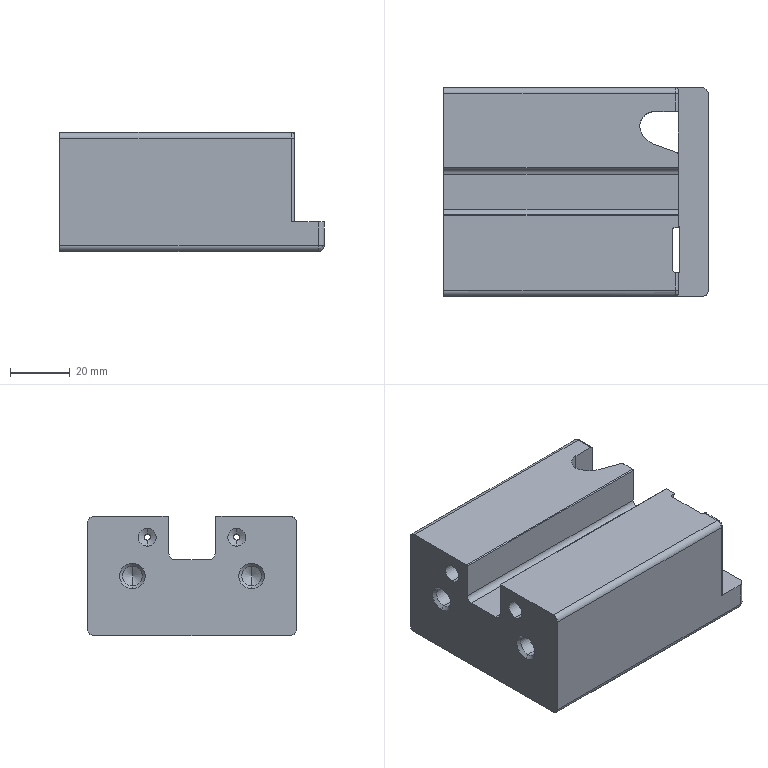Part | STEP file | LUOI CAT | 1 solid | 78 faces | box 88.8 x 70 x 40 mm | volume 196550 mm3 | cylinder 35 | plane 22 | cone 16 | spline 5 | commonest cylinder face diameters 2 x10 4 x9 6.647 x6 6 x4 0.6 x2 1 x2